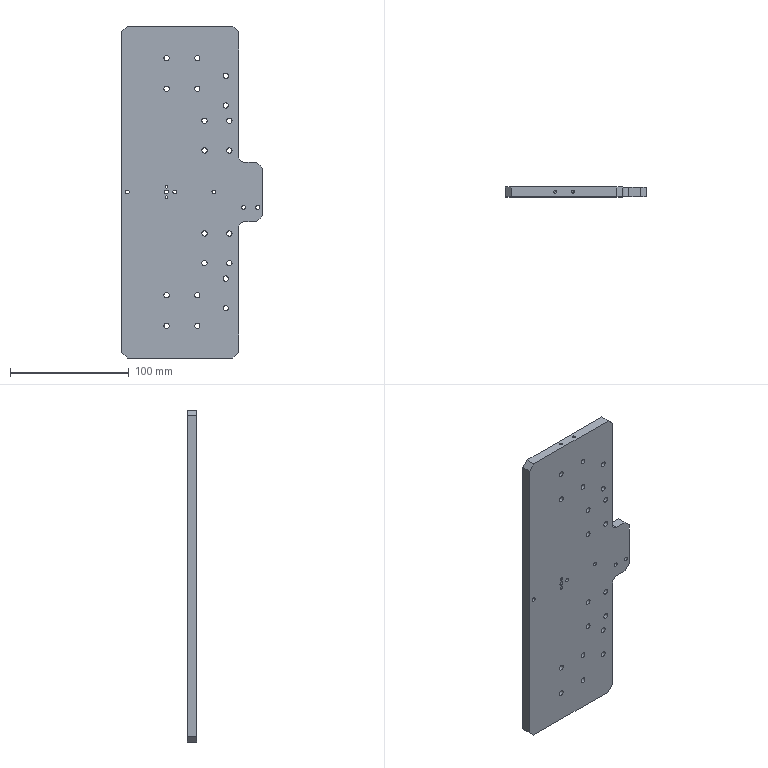Part | NX | 1 solid | 94 faces | box 119 x 8 x 280 mm | volume 222899 mm3 | cylinder 54 | plane 36 | cone 4 | commonest cylinder face diameters 4.5 x20 8 x20 2.5 x6 3.3 x6 10 x2